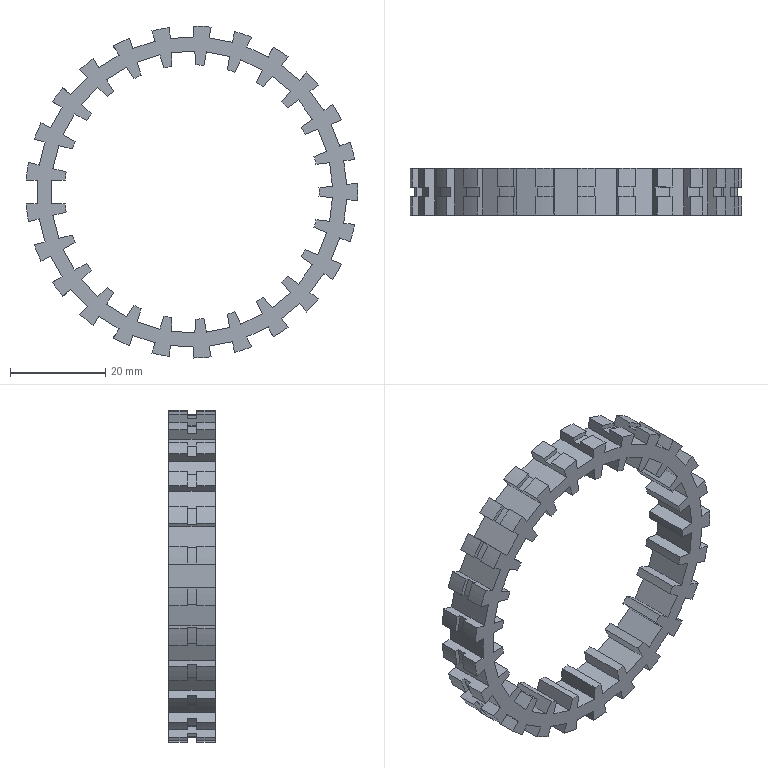Part | STEP file | Guide wheel mechanism revised.sldasm-Part-70 | 1 solid | 302 faces | box 69.71 x 9.8 x 69.797 mm | volume 8985 mm3 | plane 202 | cylinder 100 | commonest cylinder face diameters 69.8 x50 53.5 x25 68 x25